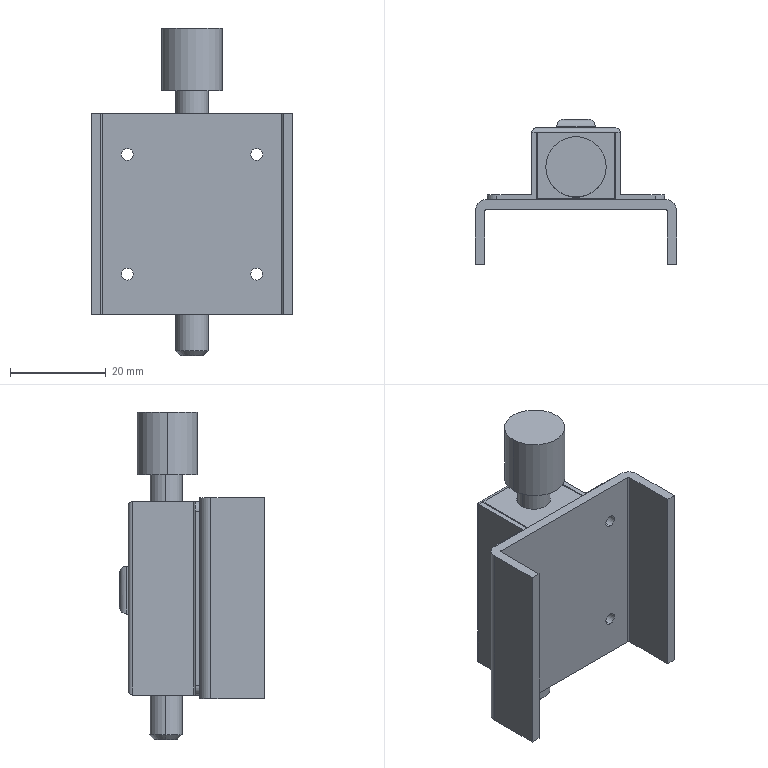Part | SolidWorks | features BaseBody 4 | 4 solids | 93 faces | box 42 x 30.3 x 68.3 mm | volume 12070 mm3 | plane 49 | cylinder 42 | cone 2 | commonest cylinder face diameters 2.5 x8 3.2 x8 0.6 x4 2 x4 3 x4 4 x4